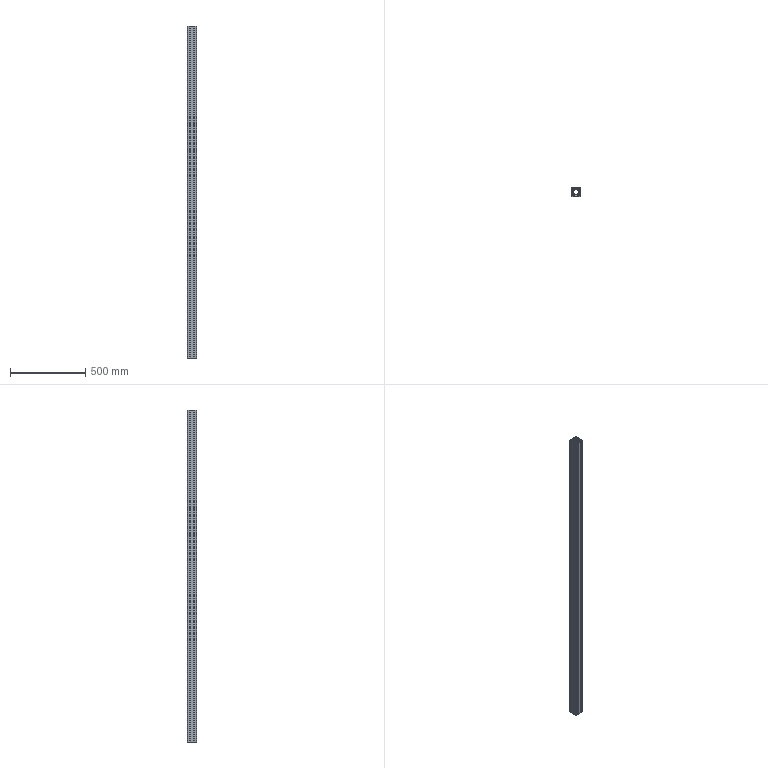Part | NX | features BREP 1 | 1 solid | 162 faces | box 60 x 60 x 2210 mm | volume 3380225 mm3 | plane 130 | cylinder 32 | commonest cylinder face diameters 2 x16 6.8 x8 4 x4 6 x4